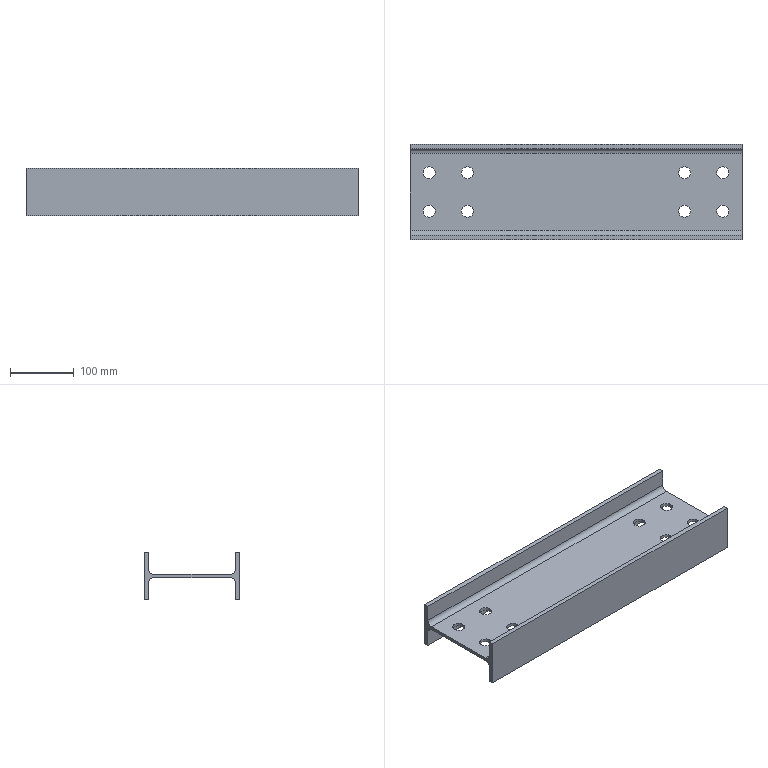Part | STEP file | 粉仓辅梁1_Default<As Machined> | 1 solid | 34 faces | box 520 x 150 x 75 mm | volume 916827 mm3 | cylinder 20 | plane 14 | commonest cylinder face diameters 19 x16 16 x4